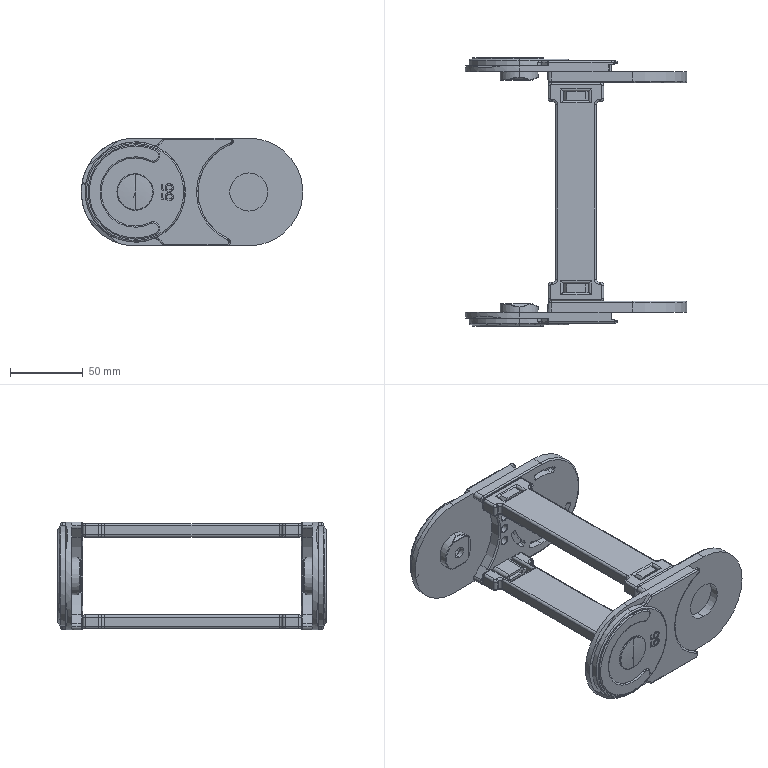Part | SolidWorks | 4 solids | 774 faces | box 152 x 185 x 74 mm | volume 243841 mm3 | plane 284 | cylinder 198 | spline 106 | torus 86 | cone 84 | sphere 16 | commonest cylinder face diameters 3 x80 4 x32 2 x24 6 x12 5 x8 9 x6